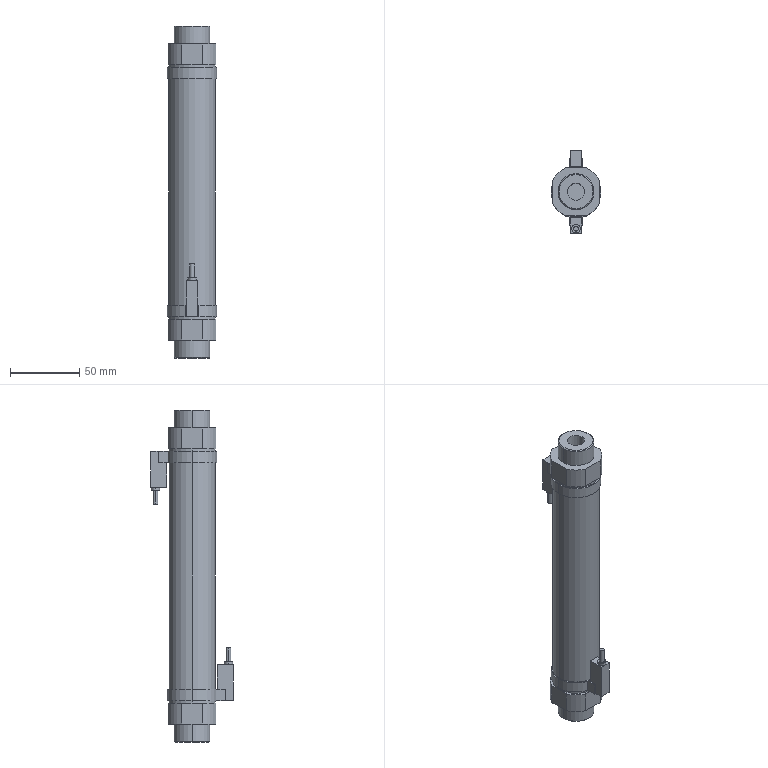Part | STEP file | body_A_CDM2B32_150_C76_0_ | 1 solid | 96 faces | box 35.8 x 59.8 x 240 mm | volume 197747 mm3 | plane 48 | cylinder 40 | cone 8 | commonest cylinder face diameters 35.8 x8 37.5 x8 33.8 x6 3.4 x4 6 x4 8.57 x4